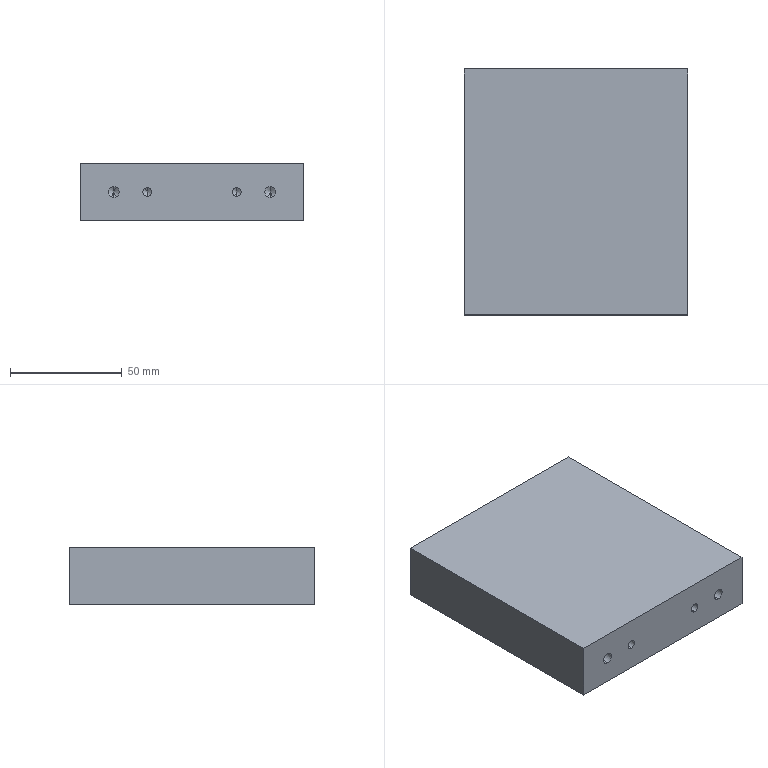Part | STEP file | PN_0020 | 1 solid | 30 faces | box 100 x 110 x 25.5 mm | volume 279122 mm3 | cylinder 12 | cone 12 | plane 6 | commonest cylinder face diameters 5 x8 4 x4